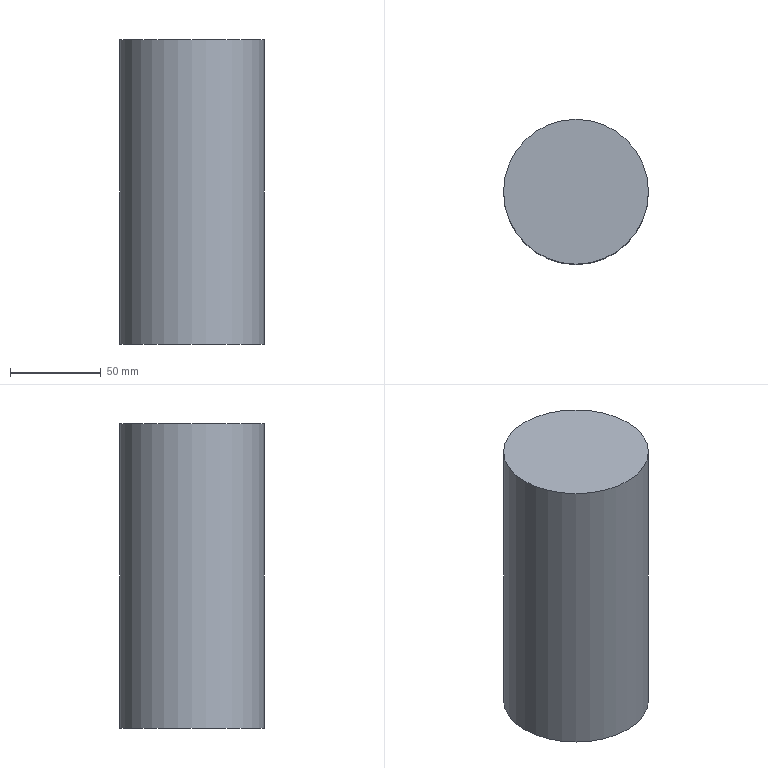Part | NX | features MAIN_BODY 2 | 1 solid | 3 faces | box 80 x 80 x 168 mm | volume 844460 mm3 | plane 2 | cylinder 1 | commonest cylinder face diameters 80 x1
STEP:
#1=CARTESIAN_POINT('',(200.,-130.,-393.));
#2=VERTEX_POINT('',#1);
#3=CARTESIAN_POINT('',(200.,-90.,-393.));
#4=DIRECTION('',(0.,0.,-1.));
#5=DIRECTION('',(0.,-1.,0.));
#6=AXIS2_PLACEMENT_3D('',#3,#4,#5);
#7=CIRCLE('',#6,40.);
#8=EDGE_CURVE('',#2,#2,#7,.T.);
#9=ORIENTED_EDGE('',*,*,#8,.F.);
#10=EDGE_LOOP('',(#9));
#11=FACE_BOUND('',#10,.T.);
#12=CARTESIAN_POINT('',(200.,-130.,-225.));
#13=VERTEX_POINT('',#12);
#14=CARTESIAN_POINT('',(200.,-90.,-225.));
#15=DIRECTION('',(0.,0.,-1.));
#16=DIRECTION('',(0.,-1.,0.));
#17=AXIS2_PLACEMENT_3D('',#14,#15,#16);
#18=CIRCLE('',#17,40.);
#19=EDGE_CURVE('',#13,#13,#18,.T.);
#20=ORIENTED_EDGE('',*,*,#19,.T.);
#21=EDGE_LOOP('',(#20));
#22=FACE_BOUND('',#21,.T.);
#23=CARTESIAN_POINT('',(200.,-90.,-393.));
#24=DIRECTION('',(0.,0.,1.));
#25=DIRECTION('',(0.,-1.,0.));
#26=AXIS2_PLACEMENT_3D('',#23,#24,#25);
#27=CYLINDRICAL_SURFACE('',#26,40.);
#28=ADVANCED_FACE('',(#11,#22),#27,.T.);
#29=ORIENTED_EDGE('',*,*,#8,.T.);
#30=EDGE_LOOP('',(#29));
#31=FACE_BOUND('',#30,.T.);
#32=CARTESIAN_POINT('',(200.,-90.,-393.));
#33=DIRECTION('',(0.,0.,-1.));
#34=DIRECTION('',(0.,1.,0.));
#35=AXIS2_PLACEMENT_3D('',#32,#33,#34);
#36=PLANE('',#35);
#37=ADVANCED_FACE('',(#31),#36,.T.);
#38=ORIENTED_EDGE('',*,*,#19,.F.);
#39=EDGE_LOOP('',(#38));
#40=FACE_BOUND('',#39,.T.);
#41=CARTESIAN_POINT('',(200.,-90.,-225.));
#42=DIRECTION('',(0.,0.,-1.));
#43=DIRECTION('',(0.,1.,0.));
#44=AXIS2_PLACEMENT_3D('',#41,#42,#43);
#45=PLANE('',#44);
#46=ADVANCED_FACE('',(#40),#45,.F.);
#47=CLOSED_SHELL('',(#28,#37,#46));
#48=MANIFOLD_SOLID_BREP('',#47);
#49=(LENGTH_UNIT()NAMED_UNIT(*)SI_UNIT(.MILLI.,.METRE.));
#50=UNCERTAINTY_MEASURE_WITH_UNIT(LENGTH_MEASURE(0.00001),#49,'','');
#51=(NAMED_UNIT(*)PLANE_ANGLE_UNIT()SI_UNIT($,.RADIAN.));
#52=(NAMED_UNIT(*)SI_UNIT($,.STERADIAN.)SOLID_ANGLE_UNIT());
#53=(GEOMETRIC_REPRESENTATION_CONTEXT(3)GLOBAL_UNCERTAINTY_ASSIGNED_CONTEXT((#50))GLOBAL_UNIT_ASSIGNED_CONTEXT((#49,#51,#52))REPRESENTATION_CONTEXT('',''));
#54=ADVANCED_BREP_SHAPE_REPRESENTATION('',(#48),#53);